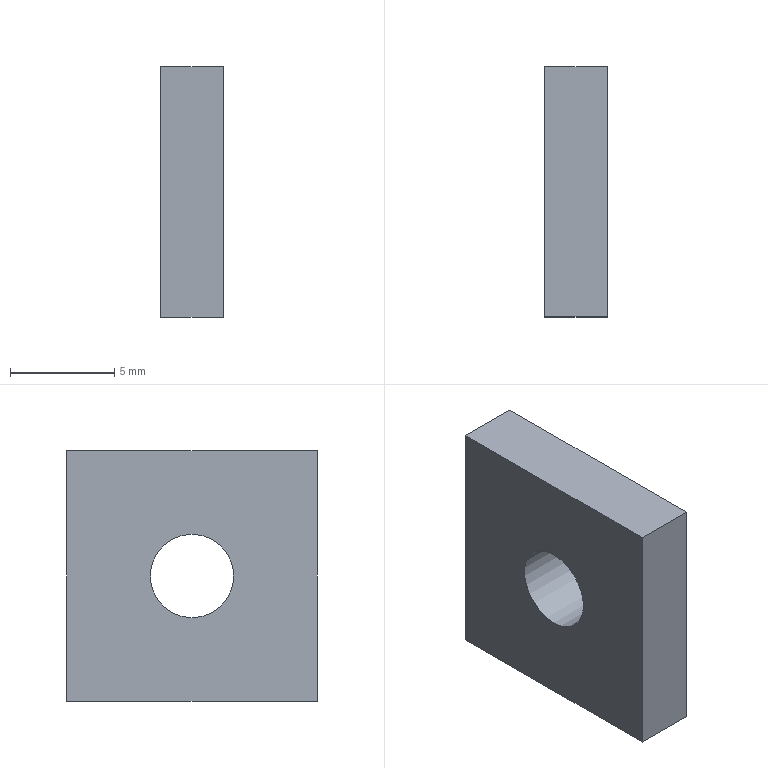Part | STEP file | solid 131 | 1 solid | 7 faces | box 3 x 12 x 12 mm | volume 394.301 mm3 | plane 6 | cylinder 1 | commonest cylinder face diameters 4 x1